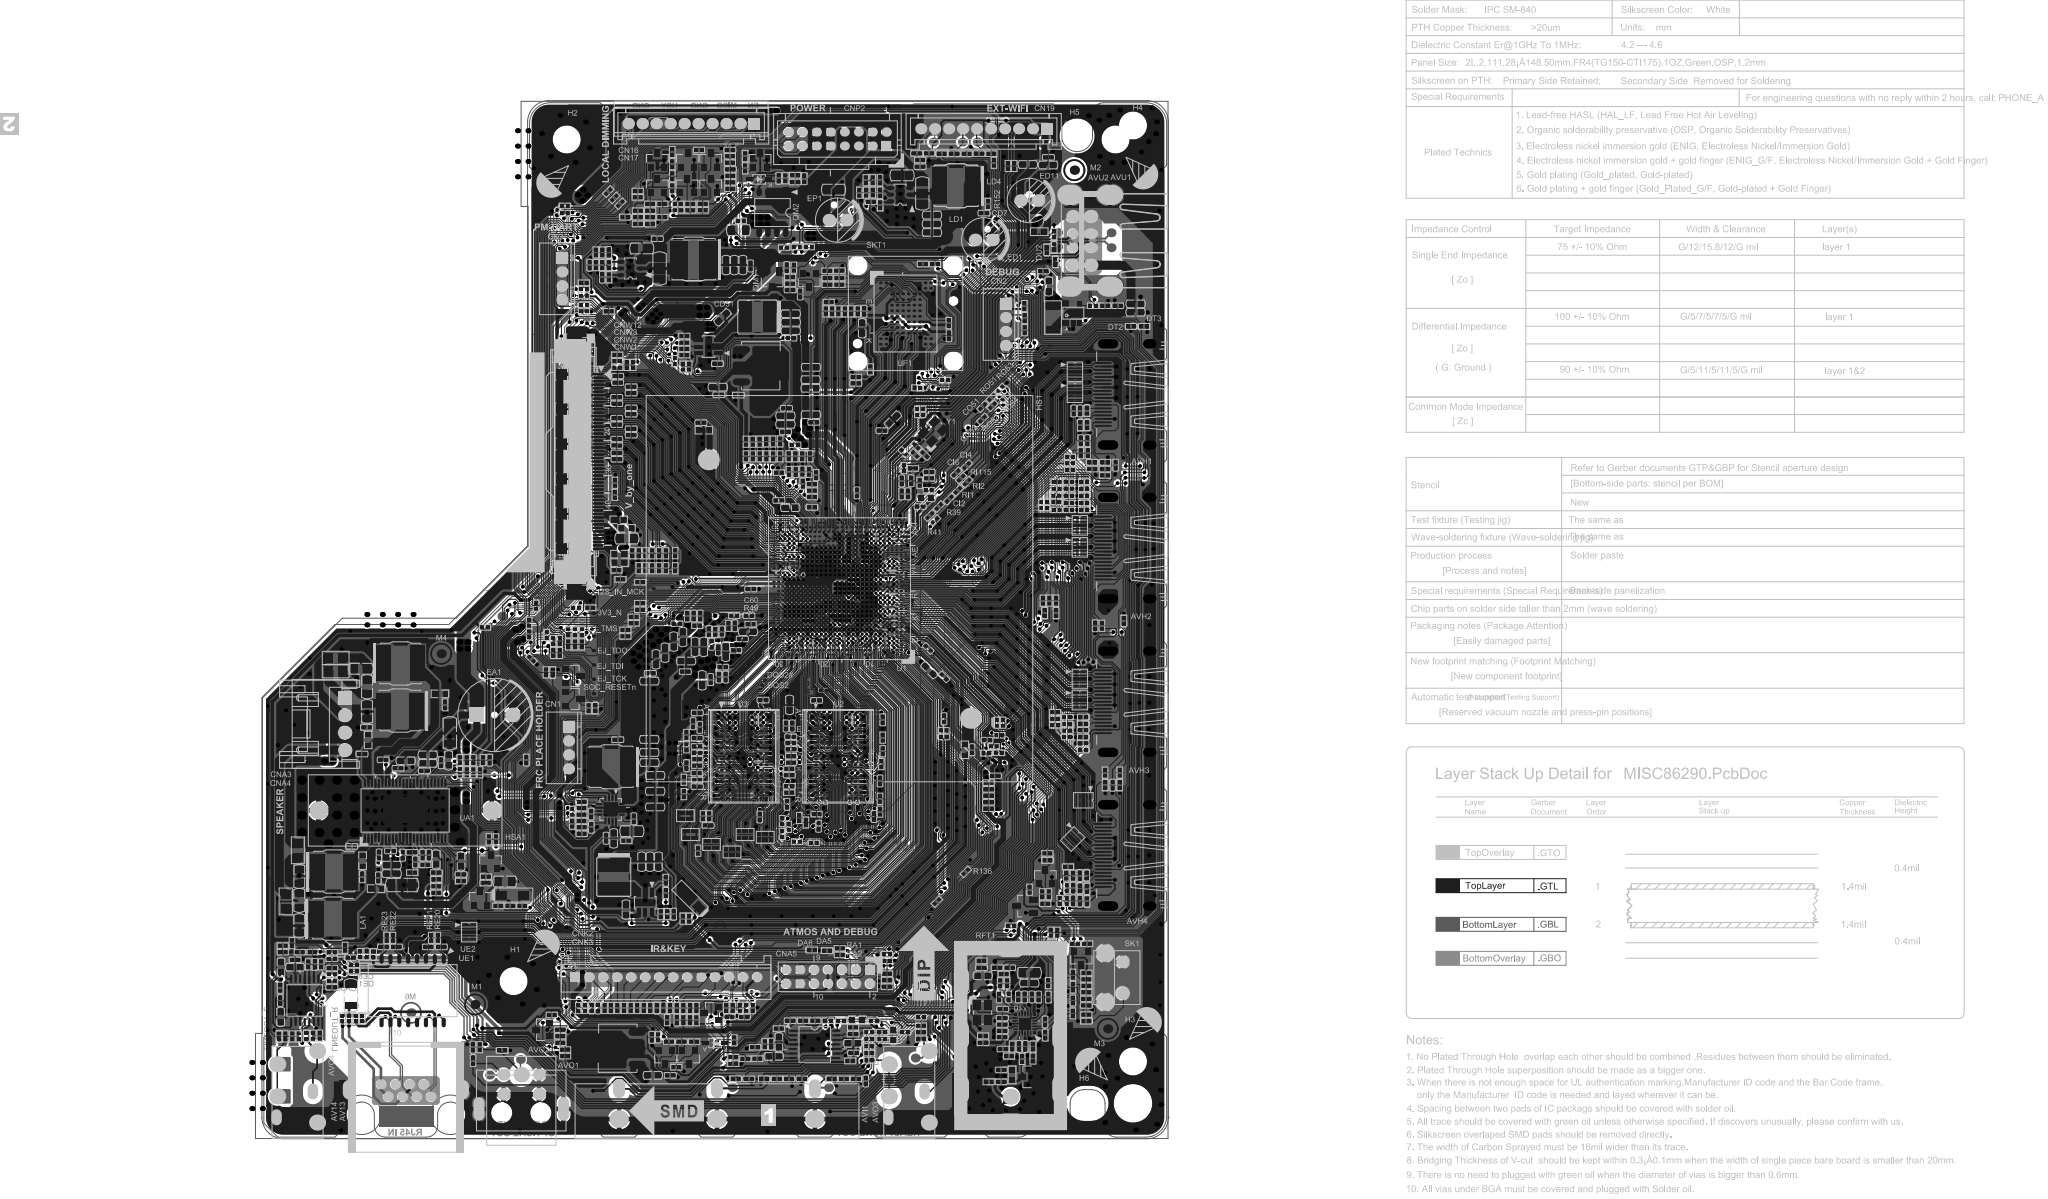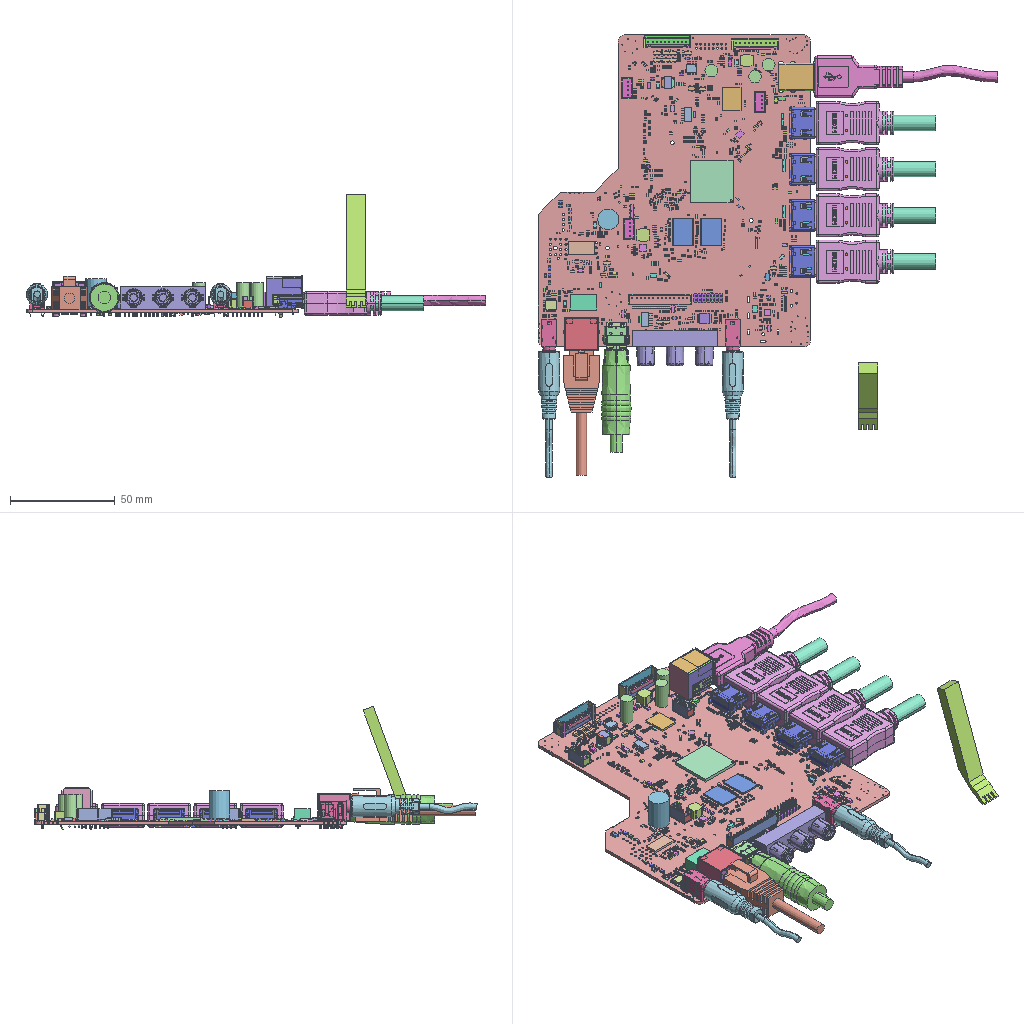Circuit board layout | Altium Designer | box 218.8 x 210.8 x 58.9 mm
Layer stack:
# Altium Designer layer stack of  (unit mm; dielectric type: 0 none, 1 core, 2 prepreg, 3 surface material)
index,name,kind,layer,copper_thickness_mm,dielectric_type,dielectric_thickness_mm,dielectric_material,dielectric_constant
0,TopPaste,other,,,,,,
1,TopOverlay,other,,,,,,
2,TopSolder,dielectric,,,3,0.0102,Solder Resist,3.5
3,TopLayer,copper,TopLayer,0.0356,,,,
4,Dielectric1,dielectric,,,1,1.5,FR-4,4.8
5,BottomLayer,copper,BottomLayer,0.0356,,,,
6,BottomSolder,dielectric,,,3,0.0102,Solder Resist,3.5
7,BottomOverlay,other,,,,,,
8,BottomPaste,other,,,,,,
# drill layer pairs: low layer,high layer
drill_pair,TopLayer,BottomLayer
Part placement, first 372 of 1027 lines:
Designator,Comment,Layer,Footprint,Center-X(mm),Center-Y(mm),Rotation
DH37,NC/TVS diode,DIO ESD,0.5pF,25V,0402 DFN,SMD,AZ5325-01F.R7G,Amazing,TopLayer,DIODE-S0402,-6.316,74.098,270
CH16,22pF-0402-NPO-¡À5%-50V,TopLayer,C0402,-7.493,96.368,90
DBS7,DOLBY PLUS,BottomLayer,DOLBY_PLUS-SILK,-603.079,-354.451,90
CO27,Ceramic capacitor,CAP MC,50V,100pF,¡À5%,NPO,0402,SMD,TP,TopLayer,C0402,-54.026,16.84,360
CO26,Ceramic capacitor,CAP MC,50V,100pF,¡À5%,NPO,0402,SMD,TP,TopLayer,C0402,-45.034,14.91,180
CO15,Ceramic capacitor,CAP MC,50V,680pF,¡À5%,NPO,0402,SMD,TP,Walsin,TopLayer,C0402,-48.628,16.84,180
RU18,4K7ohm-0402-¡À5%-1/16W,TopLayer,R0402,-31.871,108.534,180
RO58,NC/47Kohm-0402-¡À5%-1/16W,TopLayer,R0402,-42.71,14.211,180
RO57,NC/47Kohm-0402-¡À5%-1/16W,TopLayer,R0402,-55.657,15.71,360
RO56,24Kohm-0402-¡À1%-1/16W,TopLayer,R0402,-45.034,15.862,180
RO55,24Kohm-0402-¡À1%-1/16W,TopLayer,R0402,-52.178,16.84,180
RG44,100ohm-0402-¡À5%-1/16W,TopLayer,R0402,-83.547,119.291,360
RG43,100ohm-0402-¡À5%-1/16W,TopLayer,R0402,-75.489,79.616,360
R208,0ohm-0402-¡À5%-1/16W,TopLayer,R0402,-36.194,97.909,315
R207,4K7ohm-0402-¡À5%-1/16W,TopLayer,R0402,-83.845,70.701,90
R206,4K7ohm-0402-¡À5%-1/16W,TopLayer,R0402,-83.845,72.428,270
R205,100ohm-0402-¡À5%-1/16W,TopLayer,R0402,-77.597,71.857,360
R204,100ohm-0402-¡À5%-1/16W,TopLayer,R0402,-77.597,72.784,360
R203,100ohm-0402-¡À5%-1/16W,TopLayer,R0402,-76.423,73.724,360
R202,100ohm-0402-¡À5%-1/16W,TopLayer,R0402,-76.423,74.651,360
R201,100ohm-0402-¡À5%-1/16W,TopLayer,R0402,-75.489,76.606,360
R200,100ohm-0402-¡À5%-1/16W,TopLayer,R0402,-75.495,75.679,360
R31,4K7ohm-0402-¡À5%-1/16W,TopLayer,R0402,-83.553,121.574,0
R30,4K7ohm-0402-¡À5%-1/16W,TopLayer,R0402,-83.553,120.659,0
C14,0.1uF-0402-X5R-¡À20%-16V,TopLayer,C0402,-25.647,47.189,360
M6,MARK,BottomLayer,MARK,-108.28,17.958,180
M5,MARK,BottomLayer,MARK,-13.386,138.608,180
M4,MARK,TopLayer,MARK,-103.95,69.367,0
M3,MARK,TopLayer,MARK,-8.611,15.672,0
M2,MARK,TopLayer,MARK,-13.386,138.608,0
M1,MARK,TopLayer,MARK,-99.111,19.152,0
RT13,NC/0ohm-0402-PCB,TopLayer,R0402SC,-37.782,95.942,270
RT11,NC/0ohm-0402-PCB,TopLayer,R0402SC,-36.462,95.898,180
P1(用于U1上),Thermal grease,0.05g,Other,white,NULL,TopLayer,PCB_TIME,-9.804,-5.969,180
DR4,NC/TVS diode,DIO ESD,3pF,58V,0402,SMD,SDV1005H260C030YPTF,Sunlord,BottomLayer,DIODE-S0402,-37.44,68.694,180
C214,NC/10uF-0805-X5R-¡À20%-16V,BottomLayer,C0805,-55.804,76.327,270
C213,NC/0.1uF-0402-X5R-¡À20%-16V,BottomLayer,C0402,-49.581,77.114,270
C212,NC/0.1uF-0402-X5R-¡À20%-16V,BottomLayer,C0402,-47.625,76.975,270
C211,NC/10uF-0805-X5R-¡À20%-16V,BottomLayer,C0805,-47.676,89.459,225
C210,NC/0.1uF-0402-X5R-¡À20%-16V,BottomLayer,C0402,-46.228,87.122,180
C209,NC/0.1uF-0402-X5R-¡À20%-16V,BottomLayer,C0402,-46.203,88.062,180
C208,NC/10uF-0805-X5R-¡À20%-16V,BottomLayer,C0805,-59.131,73.027,90
C207,NC/0.1uF-0402-X5R-¡À20%-16V,BottomLayer,C0402,-49.454,74.701,135
C206,NC/0.1uF-0402-X5R-¡À20%-16V,BottomLayer,C0402,-50.19,73.254,270
CO25,1uF-0402-X5R-¡À20%-6.3V,TopLayer,C0402,-86.913,15.557,180
5V_M,TEST,BottomLayer,TP,-23.811,124.841,180
CU5,10uF-0603-X5R-¡À20%-6.3V,TopLayer,C0603,-4.623,119.456,360
UH3,Current-limit switch,IC OCP,2.1A,5.5V,H,SOT23-5,SMD,APL3551ABI-TRG,ANPEC,TopLayer,SOT-23-5,-13.538,118.135,360
RU6,4K7ohm-0402-¡À5%-1/16W,TopLayer,R0402,-10.719,119.202,180
RU3,4K7ohm-0402-¡À5%-1/16W,TopLayer,R0402,-8.966,119.202,360
FU1,NC/Resettable fuse,FUSE PTC,1.1A,6V,1206,SMD,TP,TLC,TopLayer,FUSE1.1A-S,-16.434,117.5,270
CU4,0.1uF-0402-X5R-¡À20%-16V,TopLayer,C0402,-17.805,124.155,360
CU3,NC/10uF-0603-X5R-¡À20%-6.3V,TopLayer,C0603,-17.043,121.971,270
CU2,10uF-0603-X5R-¡À20%-6.3V,TopLayer,C0603,-4.623,118.262,360
RM4,1Kohm-0402-¡À5%-1/16W,TopLayer,R0402,-54.038,122.365,360
R73,100ohm-0402-¡À5%-1/16W,TopLayer,R0402,-35.052,125.159,0
R72,100ohm-0402-¡À5%-1/16W,TopLayer,R0402,-33.325,125.171,360
CM4,0.022uF-0402-X7R-¡À10%-16V,TopLayer,C0402,-54.534,124.651,90
RH16,100ohm-0402-¡À5%-1/16W,TopLayer,R0402,-17.678,91.11,180
RH15,100ohm-0402-¡À5%-1/16W,TopLayer,R0402,-17.678,90.195,180
RH14,47Kohm-0402-¡À5%-1/16W,TopLayer,R0402,-15.951,91.11,180
RH13,47Kohm-0402-¡À5%-1/16W,TopLayer,R0402,-15.951,92.024,180
DH14,NC/TVS diode,DIO ESD,0.5pF,25V,0402 DFN,SMD,AZ5325-01F.R7G,Amazing,TopLayer,DIODE-S0402,-11.989,90.957,360
DH13,NC/TVS diode,DIO ESD,0.5pF,25V,0402 DFN,SMD,AZ5325-01F.R7G,Amazing,TopLayer,DIODE-S0402,-11.989,91.999,360
DH12,NC/TVS diode,DIO ESD,0.5pF,25V,0402 DFN,SMD,AZ5325-01F.R7G,Amazing,TopLayer,DIODE-S0402,-11.989,93.015,360
DH11,NC/TVS diode,DIO ESD,0.5pF,25V,0402 DFN,SMD,AZ5325-01F.R7G,Amazing,TopLayer,DIODE-S0402,-11.989,94.005,360
CH14,NC/22pF-0402-NPO-¡À5%-50V,TopLayer,C0402,-14.173,90.958,360
CH13,NC/22pF-0402-NPO-¡À5%-50V,TopLayer,C0402,-14.173,91.999,360
CH12,220pF-0402-NPO-¡À5%-50V,TopLayer,C0402,-14.173,93.015,360
CH11,220pF-0402-NPO-¡À5%-50V,TopLayer,C0402,-14.173,94.006,360
CVBSOUT1,TEST,BottomLayer,TP-20,-33.731,88.29,90
DQS3,TEST,BottomLayer,TP-20,-59.483,59.49,90
DQS3#,TEST,BottomLayer,TP-20,-59.483,60.29,90
DQS2,TEST,TopLayer,TP-20,-58.115,64.846,90
DQS2#,TEST,TopLayer,TP-20,-57.709,65.608,90
DQS1,TEST,BottomLayer,TP-20,-45.983,59.49,90
DQS1#,TEST,BottomLayer,TP-20,-45.983,60.29,90
DQS0,TEST,TopLayer,TP-20,-48.844,64.135,90
DQS0#,TEST,TopLayer,TP-20,-49.733,64.135,90
RR11,33ohm-0402-¡À5%-1/16W,TopLayer,R0402,-62.027,14.021,270
DI1,NC/TVS diode,DIO ESD,3pF,58V,0402,SMD,SDV1005H260C030YPTF,Sunlord,TopLayer,DIODE-S0402,-61.849,8.509,360
AV_L,TEST,BottomLayer,TP,-62.319,7.264,180
RP14,Resistor array,RES ARRAY,1/16W,4¡Á75ohm,¡À5%,0402,SMD,TopLayer,RA0402-MSD6886,-62.358,40.99,270
RK13,NC/33Kohm-0402-¡À5%-1/16W,TopLayer,R0402,-62.268,18.669,270
RO19,NC/?,TopLayer,R0402,-62.172,11.608,180
C59,Ceramic capacitor,CAP MC,50V,1000pF,¡À20%,X7R,0402,SMD,TP,TopLayer,C0402,-61.951,73.391,90
R45,Thick-film resistor,RES,1/16W,10Kohm,¡À5%,0402,SMD,TopLayer,R0402,-62.038,74.829,360
R48,Thick-film resistor,RES,1/16W,240ohm,¡À1%,0402,SMD,TopLayer,R0402,-61.784,69.851,360
MOD_1V2,TEST,BottomLayer,TP,-60.985,94.288,90
U1,TV main chip,IC Main Chip,MSDURN1801-R-00E3,64bit,Multi-Core,BGA758,SMD,Mstar,TopLayer,BGA758/0.65,-46.983,78.69,180
H6,Location hole,TopLayer,ASSE5.0C-3,-5.093,5.292,0
RH38,100ohm-0402-¡À5%-1/16W,TopLayer,R0402,-8.986,52.362,90
DR5,NC/TVS diode,DIO ESD,3pF,58V,0402,SMD,SDV1005H260C030YPTF,Sunlord,TopLayer,DIODE-S0402,-50.902,90.351,180
DH35,NC/TVS diode,DIO ESD,0.5pF,25V,0402 DFN,SMD,AZ5325-01F.R7G,Amazing,TopLayer,DIODE-S0402,-8.973,50.559,90
3V3_STB,TEST,BottomLayer,TP,-94.297,70.968,180
RU5,10Kohm-0402-¡À5%-1/16W,TopLayer,R0402,-51.181,97.638,270
CL25,NC/0.1uF-0402-X5R-¡À20%-16V,TopLayer,C0402,-64.237,106.451,360
CL13,Ceramic capacitor,CAP MC,6.3V,10uF,¡À20%,X5R,0603,SMD,TP,TopLayer,C0603,-64.389,107.544,360
C35,Ceramic capacitor,CAP MC,6.3V,10uF,¡À20%,X5R,0603,SMD,TP,TopLayer,C0603,-54.712,102.21,360
C34,0.1uF-0402-X5R-¡À20%-16V,TopLayer,C0402,-54.572,104.508,180
C33,0.1uF-0402-X5R-¡À20%-16V,TopLayer,C0402,-54.712,101.143,180
C32,0.1uF-0402-X5R-¡À20%-16V,TopLayer,C0402,-53.365,99.289,180
C26,0.1uF-0402-X5R-¡À20%-16V,TopLayer,C0402,-55.651,91.316,180
C25,Ceramic capacitor,CAP MC,6.3V,10uF,¡À20%,X5R,0603,SMD,TP,TopLayer,C0603,-54.026,90.284,360
C20,0.1uF-0402-X5R-¡À20%-16V,TopLayer,C0402,-50.646,102.502,360
MCP_TEST,TEST,BottomLayer,TP-20,-52.172,81.255,180
R26,NC/Thick-film resistor,RES,1/16W,4.7Kohm,¡À5%,0402,SMD,TopLayer,R0402,-59.379,97.627,270
R23,Thick-film resistor,RES,1/16W,4.7Kohm,¡À5%,0402,SMD,TopLayer,R0402,-58.388,97.627,270
R22,Thick-film resistor,RES,1/16W,4.7Kohm,¡À5%,0402,SMD,TopLayer,R0402,-56.458,97.627,270
R21,Thick-film resistor,RES,1/16W,4.7Kohm,¡À5%,0402,SMD,TopLayer,R0402,-60.369,97.627,270
R20,Thick-film resistor,RES,1/16W,4.7Kohm,¡À5%,0402,SMD,TopLayer,R0402,-57.423,97.627,270
R18,Thick-film resistor,RES,1/16W,4.7Kohm,¡À5%,0402,SMD,TopLayer,R0402,-59.404,99.733,90
R15,NC/Thick-film resistor,RES,1/16W,4.7Kohm,¡À5%,0402,SMD,TopLayer,R0402,-58.414,99.733,90
R14,NC/Thick-film resistor,RES,1/16W,4.7Kohm,¡À5%,0402,SMD,TopLayer,R0402,-56.483,99.758,90
R13,NC/Thick-film resistor,RES,1/16W,4.7Kohm,¡À5%,0402,SMD,TopLayer,R0402,-60.369,99.733,90
R12,NC/Thick-film resistor,RES,1/16W,4.7Kohm,¡À5%,0402,SMD,TopLayer,R0402,-57.448,99.758,90
R10,Thick-film resistor,RES,1/16W,4.7Kohm,¡À5%,0402,SMD,TopLayer,R0402,-55.467,97.632,270
R6,NC/Thick-film resistor,RES,1/16W,4.7Kohm,¡À5%,0402,SMD,TopLayer,R0402,-55.467,99.764,90
R27,NC/Thick-film resistor,RES,1/16W,4.7Kohm,¡À5%,0402,SMD,TopLayer,R0402,-52.248,93.726,270
R25,Thick-film resistor,RES,1/16W,4.7Kohm,¡À5%,0402,SMD,TopLayer,R0402,-52.273,95.453,270
R24,Thick-film resistor,RES,1/16W,4.7Kohm,¡À5%,0402,SMD,TopLayer,R0402,-53.264,95.402,270
R19,Thick-film resistor,RES,1/16W,4.7Kohm,¡À5%,0402,SMD,TopLayer,R0402,-50.927,93.65,360
R17,NC/Thick-film resistor,RES,1/16W,4.7Kohm,¡À5%,0402,SMD,TopLayer,R0402,-51.333,95.428,90
R16,NC/Thick-film resistor,RES,1/16W,4.7Kohm,¡À5%,0402,SMD,TopLayer,R0402,-52.299,97.638,90
R11,Thick-film resistor,RES,1/16W,4.7Kohm,¡À5%,0402,SMD,TopLayer,R0402,-50.927,91.821,180
R9,Thick-film resistor,RES,1/16W,4.7Kohm,¡À5%,0402,SMD,TopLayer,R0402,-54.229,95.402,270
R8,NC/Thick-film resistor,RES,1/16W,4.7Kohm,¡À5%,0402,SMD,TopLayer,R0402,-55.651,95.301,360
R7,NC/Thick-film resistor,RES,1/16W,4.7Kohm,¡À5%,0402,SMD,TopLayer,R0402,-50.927,92.735,360
R5,NC/Thick-film resistor,RES,1/16W,4.7Kohm,¡À5%,0402,SMD,TopLayer,R0402,-53.289,97.638,90
R4,Thick-film resistor,RES,1/16W,4.7Kohm,¡À5%,0402,SMD,TopLayer,R0402,-54.254,97.638,90
RO1,100ohm-0402-¡À5%-1/16W,TopLayer,R0402,-24.917,56.096,360
R123,Thick-film resistor,RES,1/16W,1Kohm,¡À5%,0402,SMD,TopLayer,R0402,-32.087,58.395,180
CO3,33pF-0402-NPO-¡À5%-50V,TopLayer,C0402,-25.889,56.998,360
C174,Ceramic capacitor,CAP MC,50V,330pF,¡À5%,NPO,0402,SMD,TP,TopLayer,C0402,-32.087,57.455,180
AV_R,TEST,BottomLayer,TP,-48.539,7.239,180
R118,Thick-film resistor,RES,1/16W,620ohm,¡À1%,0402,SMD,TopLayer,R0402,-55.183,45.407,90
R108,Thick-film resistor,RES,1/16W,10Kohm,¡À5%,0402,SMD,TopLayer,R0402,-54.166,49.49,180
R100,Thick-film resistor,RES,1/16W,240ohm,¡À1%,0402,SMD,TopLayer,R0402,-54.166,52.89,180
R67,Thick-film resistor,RES,1/16W,10Kohm,¡À1%,0402,SMD,TopLayer,R0402,-41.183,48.607,270
R66,Thick-film resistor,RES,1/16W,10Kohm,¡À1%,0402,SMD,TopLayer,R0402,-41.183,46.773,270
R65,Thick-film resistor,RES,1/16W,620ohm,¡À1%,0402,SMD,TopLayer,R0402,-55.183,43.573,90
R64,Thick-film resistor,RES,1/16W,240ohm,¡À1%,0402,SMD,TopLayer,R0402,-40.983,53.573,90
R63,Thick-film resistor,RES,1/16W,10Kohm,¡À5%,0402,SMD,TopLayer,R0402,-50.258,46.398,180
R62,Thick-film resistor,RES,1/16W,10Kohm,¡À5%,0402,SMD,TopLayer,R0402,-40.808,57.357,270
R59,Thick-film resistor,RES,1/16W,75ohm,¡À5%,0402,SMD,TopLayer,R0402,-50.666,42.29,180
R56,Thick-film resistor,RES,1/16W,22ohm,¡À5%,0402,SMD,TopLayer,R0402,-53.066,42.49,180
R55,Thick-film resistor,RES,1/16W,75ohm,¡À5%,0402,SMD,TopLayer,R0402,-52.733,45.857,270
R54,Thick-film resistor,RES,1/16W,75ohm,¡À5%,0402,SMD,TopLayer,R0402,-51.783,45.207,270
R53,Thick-film resistor,RES,1/16W,22ohm,¡À5%,0402,SMD,TopLayer,R0402,-54.262,44.594,270
R52,Thick-film resistor,RES,1/16W,22ohm,¡À5%,0402,SMD,TopLayer,R0402,-40.808,55.407,270
R51,Thick-film resistor,RES,1/16W,22ohm,¡À5%,0402,SMD,TopLayer,R0402,-53.9,53.79,180
R50,Thick-film resistor,RES,1/16W,22ohm,¡À5%,0402,SMD,TopLayer,R0402,-53.9,54.69,180
R49,Thick-film resistor,RES,1/16W,240ohm,¡À1%,0402,SMD,TopLayer,R0402,-59.702,73.61,360
C100,Ceramic capacitor,CAP MC,50V,1000pF,¡À20%,X7R,0402,SMD,TP,TopLayer,C0402,-54.166,51.99,180
C99,Ceramic capacitor,CAP MC,50V,1000pF,¡À20%,X7R,0402,SMD,TP,TopLayer,C0402,-41.183,51.173,90
C98,Ceramic capacitor,CAP MC,50V,1000pF,¡À20%,X7R,0402,SMD,TP,TopLayer,C0402,-53.951,56.59,360
C97,Ceramic capacitor,CAP MC,16V,0.1uF,¡À20%,X5R,0402,SMD,TP,TopLayer,C0402,-49.983,44.673,90
C96,NC/Ceramic capacitor,CAP MC,16V,0.1uF,¡À20%,X5R,0402,SMD,TP,BottomLayer,C0402,-50.383,51.515,270
C95,NC/Ceramic capacitor,CAP MC,16V,0.1uF,¡À20%,X5R,0402,SMD,TP,BottomLayer,C0402,-45.483,56.49,270
C93,NC/Ceramic capacitor,CAP MC,16V,0.1uF,¡À20%,X5R,0402,SMD,TP,BottomLayer,C0402,-57.683,54.965,90
C92,NC/Ceramic capacitor,CAP MC,16V,0.1uF,¡À20%,X5R,0402,SMD,TP,BottomLayer,C0402,-57.683,57.065,90
C91,NC/Ceramic capacitor,CAP MC,16V,0.1uF,¡À20%,X5R,0402,SMD,TP,BottomLayer,C0402,-57.651,50.665,90
C90,NC/Ceramic capacitor,CAP MC,16V,0.1uF,¡À20%,X5R,0402,SMD,TP,BottomLayer,C0402,-49.74,49.203,180
C83,NC/Ceramic capacitor,CAP MC,16V,0.1uF,¡À20%,X5R,0402,SMD,TP,BottomLayer,C0402,-58.283,48.673,90
C76,Ceramic capacitor,CAP MC,16V,0.1uF,¡À20%,X5R,0402,SMD,TP,TopLayer,C0402,-57.916,62.74,180
C74,Ceramic capacitor,CAP MC,16V,0.1uF,¡À20%,X5R,0402,SMD,TP,TopLayer,C0402,-42.058,46.073,90
C73,Ceramic capacitor,CAP MC,16V,0.1uF,¡À20%,X5R,0402,SMD,TP,TopLayer,C0402,-53.9,55.69,360
C70,Ceramic capacitor,CAP MC,16V,0.1uF,¡À20%,X5R,0402,SMD,TP,TopLayer,C0402,-40.808,59.923,90
C67,Ceramic capacitor,CAP MC,16V,0.1uF,¡À20%,X5R,0402,SMD,TP,TopLayer,C0402,-50.266,62.69,180
C66,Ceramic capacitor,CAP MC,16V,0.1uF,¡À20%,X5R,0402,SMD,TP,TopLayer,C0402,-53.73,59.028,90
C65,Ceramic capacitor,CAP MC,16V,0.1uF,¡À20%,X5R,0402,SMD,TP,TopLayer,C0402,-54.633,59.028,90
C60,Ceramic capacitor,CAP MC,16V,0.1uF,¡À20%,X5R,0402,SMD,TP,TopLayer,C0402,-59.949,74.817,180
C58,NC/Ceramic capacitor,CAP MC,16V,0.1uF,¡À20%,X5R,0402,SMD,TP,TopLayer,C0402,-60.884,71.488,360
C51,Ceramic capacitor,CAP MC,6.3V,10uF,¡À20%,X5R,0603,SMD,TP,TopLayer,C0603,-54.128,62.051,270
C50,Ceramic capacitor,CAP MC,6.3V,0.47uF,¡À10%,X5R,0402,SMD,TP,TopLayer,C0402,-58.393,45.993,270
C46,NC/Ceramic capacitor,CAP MC,6.3V,0.47uF,¡À10%,X5R,0402,SMD,TP,BottomLayer,C0402,-45.866,73.49,360
C42,0.1uF-0402-X5R-¡À20%-16V,TopLayer,C0402,-54.483,47.807,90
C39,Ceramic capacitor,CAP MC,6.3V,10uF,¡À20%,X5R,0603,SMD,TP,TopLayer,C0603,-60.071,72.53,360
UH22,NC/TVS diode,DIO ESD,0.4pF,19V,DFN2510-10L,SMD,ESD5304D-10/TR,Willsemi,TopLayer,RCL0524P,-12.598,62.738,270
UA2,Audio amplifier,IC Headphone AMP,Class AB,2¡Á20mW@2.3V@32ohm,TSSOP-14,SMD,AD22653B-QH14NAR,ESMT,TopLayer,SSOP14/0.65-1,-50.521,13.437,270
RO30,4K7ohm-0402-¡À5%-1/16W,TopLayer,R0402,-59.055,13.03,360
RO29,0ohm-0402-¡À5%-1/16W,TopLayer,R0402,-57.683,13.462,90
RO25,1Kohm-0402-¡À5%-1/16W,TopLayer,R0402,-42.71,12.192,360
RO24,1Kohm-0402-¡À5%-1/16W,TopLayer,R0402,-35.316,15.186,360
RO23,10Kohm-0402-¡À5%-1/16W,TopLayer,R0402,-86.226,12.7,180
RO22,1Kohm-0402-¡À5%-1/16W,TopLayer,R0402,-88.145,17.653,360
RO21,30Kohm-0402-¡À1%-1/16W,TopLayer,R0402,-58.725,11.405,360
RO20,1Kohm-0402-¡À5%-1/16W,TopLayer,R0402,-60.445,11.379,360
RO16,5R1ohm-0402-¡À5%-1/16W,TopLayer,R0402,-42.71,13.157,360
RO15,5R1ohm-0402-¡À5%-1/16W,TopLayer,R0402,-35.316,16.138,360
RO14,10Kohm-0402-¡À5%-1/16W,TopLayer,R0402,-42.71,15.186,180
RO12,10Kohm-0402-¡À5%-1/16W,TopLayer,R0402,-40.856,14.211,180
RO11,10Kohm-0402-¡À5%-1/16W,TopLayer,R0402,-46.749,16.84,180
RK23,22ohm-0402-¡À5%-1/16W,TopLayer,R0402,-62.713,17.374,360
RK14,NC/510ohm-0402-¡À1%-1/16W,TopLayer,R0402,-61.227,18.682,90
LO2,Ferrite bead,BEAD,120ohm,0402,500mA,SMD,TP,GZ1005U121CTF,Sunlord,TopLayer,L0402,-45.441,11.074,180
H3,Location hole,TopLayer,ASSE3.5C-3,-5.1,8.216,0
DO12,NC/NC?,TopLayer,DIODE-S0402,-42.697,11.176,360
DO11,NC/NC?,TopLayer,DIODE-S0402,-35.306,14.211,360
CO24,NC/0.1uF-0402-X5R-¡À20%-16V,TopLayer,C0402,-91.77,54.14,90
CO21,0.1uF-0402-X5R-¡À20%-16V,TopLayer,C0402,-44.958,12.217,360
CO20,10uF-0603-X5R-¡À20%-6.3V,TopLayer,C0603,-45.034,13.589,360
CO19,10uF-0603-X5R-¡À20%-6.3V,TopLayer,C0603,-56.388,11.709,180
CO18,0.1uF-0402-X5R-¡À20%-16V,TopLayer,C0402,-56.744,13.462,90
CO16,Ceramic capacitor,CAP MC,50V,680pF,¡À5%,NPO,0402,SMD,TP,Walsin,TopLayer,C0402,-40.85,15.185,180
CO14,Ceramic capacitor,CAP MC,6.3V,10uF,¡À20%,X5R,0603,SMD,TP,TopLayer,C0603,-39.256,14.757,90
CO13,Ceramic capacitor,CAP MC,6.3V,10uF,¡À20%,X5R,0603,SMD,TP,TopLayer,C0603,-44.417,16.98,360
CO12,NC/000pF-0402-X7R-¡À10%-50V,TopLayer,C0402,-37.599,15.185,180
CO11,NC/1000pF-0402-X7R-¡À10%-50V,TopLayer,C0402,-42.031,16.841,360
CNA5,Gold-plated pin,pin connector,2¡Á7Pin,D,D2.0,L=2.6mm,DIP,LD,TopLayer,SIP2*7/2.0D,-48.641,23.13,360
CK8,Ceramic capacitor,CAP MC,50V,1000pF,¡À20%,X7R,0402,SMD,TP,TopLayer,C0402,-60.579,17.374,180
CK7,NC/1000pF-0402-X7R-¡À10%-50V,TopLayer,C0402,-59.411,18.682,90
C24,1uF-0402-X5R-¡À20%-6.3V,TopLayer,C0402,-32.017,66.065,315
U2,DDR chip,IC DDR3,DDR3,2133M,16bit,256MB,2Gb,FBGA96,SMD,K4B2G1646F-BCNB,Samsung,TopLayer,BGA96/0.8-1,-47.183,54.69,360
RP16,Resistor array,RES ARRAY,1/16W,4¡Á75ohm,¡À5%,0402,SMD,TopLayer,RA0402-MSD6886,-57.608,43.09,270
RP13,Resistor array,RES ARRAY,1/16W,4¡Á75ohm,¡À5%,0402,SMD,TopLayer,RA0402-MSD6886,-60.483,43.49,270
C85,NC/Ceramic capacitor,CAP MC,16V,0.1uF,¡À20%,X5R,0402,SMD,TP,BottomLayer,C0402,-42.266,58.309,180
C88,NC/Ceramic capacitor,CAP MC,16V,0.1uF,¡À20%,X5R,0402,SMD,TP,BottomLayer,C0402,-41.516,49.19,180
C81,Ceramic capacitor,CAP MC,16V,0.1uF,¡À20%,X5R,0402,SMD,TP,TopLayer,C0402,-54.166,50.39,180
C82,Ceramic capacitor,CAP MC,16V,0.1uF,¡À20%,X5R,0402,SMD,TP,TopLayer,C0402,-53.951,57.5,360
QO21,General-purpose transistor,Dynatron,NPN,0.2A,40V,60-300,SOT-23,KMBT3904,KEXIN,TopLayer,SOT-23,-89.472,15.545,270
RO26,10Kohm-0402-¡À5%-1/16W,TopLayer,R0402,-35.306,17.335,360
RO27,4K7ohm-0402-¡À5%-1/16W,TopLayer,R0402,-86.913,14.618,360
RO28,NC/?,TopLayer,R0402,-86.913,13.679,180
CI1,NC/56pF-0402-NPO-¡À5%-50V,TopLayer,C0402,-59.969,8.509,180
CI3,NC/56pF-0402-NPO-¡À5%-50V,TopLayer,C0402,-52.356,8.509,180
CI5,NC/56pF-0402-NPO-¡À5%-50V,TopLayer,C0402,-43.231,8.204,90
DI2,NC/TVS diode,DIO ESD,3pF,58V,0402,SMD,SDV1005H260C030YPTF,Sunlord,TopLayer,DIODE-S0402,-57.76,8.509,360
DI3,NC/TVS diode,DIO ESD,3pF,58V,0402,SMD,SDV1005H260C030YPTF,Sunlord,TopLayer,DIODE-S0402,-48.082,8.509,180
RI3,10Kohm-0402-¡À5%-1/16W,TopLayer,R0402,-55.931,8.509,360
RI4,18Kohm-0402-¡À1%-1/16W,TopLayer,R0402,-54.185,8.509,180
RI5,18Kohm-0402-¡À1%-1/16W,TopLayer,R0402,-44.628,8.509,180
RI6,10Kohm-0402-¡À5%-1/16W,TopLayer,R0402,-46.355,8.509,360
YT2,24MHz-¡À20ppm-16pF-3.2*2.5-SMD,TopLayer,XTAL-S-3,-26.518,17.983,270
DT3,NC/TVS diode,DIO ESD,3pF,58V,0402,SMD,SDV1005H260C030YPTF,Sunlord,TopLayer,DIODE-S0402,-3.404,116.23,180
DT2,NC/TVS diode,DIO ESD,3pF,58V,0402,SMD,SDV1005H260C030YPTF,Sunlord,TopLayer,DIODE-S0402,-5.283,116.23,360
CT40,Ceramic capacitor,CAP MC,50V,12pF,¡À5%,NPO,0402,SMD,TP,TopLayer,C0402,-23.682,17.218,360
CT39,Ceramic capacitor,CAP MC,50V,12pF,¡À5%,NPO,0402,SMD,TP,TopLayer,C0402,-23.645,18.502,180
3V3_Tun,TEST,BottomLayer,TP,-39.802,18.136,315
CH15,22pF-0402-NPO-¡À5%-50V,TopLayer,C0402,-7.925,50.546,90
CH21,220pF-0402-NPO-¡À5%-50V,TopLayer,C0402,-14.376,57.455,360
CH22,220pF-0402-NPO-¡À5%-50V,TopLayer,C0402,-12.141,56.54,180
CH23,NC/22pF-0402-NPO-¡À5%-50V,TopLayer,C0402,-12.141,58.42,180
CH24,NC/22pF-0402-NPO-¡À5%-50V,TopLayer,C0402,-14.376,60.3,360
CH31,220pF-0402-NPO-¡À5%-50V,TopLayer,C0402,-12.598,33.941,270
CH32,220pF-0402-NPO-¡À5%-50V,TopLayer,C0402,-13.564,33.985,90
CH33,NC/22pF-0402-NPO-¡À5%-50V,TopLayer,C0402,-13.538,35.814,270
CH34,NC/22pF-0402-NPO-¡À5%-50V,TopLayer,C0402,-12.598,37.617,270
CR1,1uF-0402-X5R-¡À20%-6.3V,TopLayer,C0402,-11.671,19.952,360
CR2,0.1uF-0402-X5R-¡À20%-16V,TopLayer,C0402,-22.428,30.429,360
CR3,0.1uF-0402-X5R-¡À20%-16V,TopLayer,C0402,-13.589,21.615,90
CR4,0.1uF-0402-X5R-¡À20%-16V,TopLayer,C0402,-11.671,19.012,180
DH21,NC/TVS diode,DIO ESD,0.5pF,25V,0402 DFN,SMD,AZ5325-01F.R7G,Amazing,TopLayer,DIODE-S0402,-12.141,55.601,360
DH22,NC/TVS diode,DIO ESD,0.5pF,25V,0402 DFN,SMD,AZ5325-01F.R7G,Amazing,TopLayer,DIODE-S0402,-12.141,57.429,360
DH23,NC/TVS diode,DIO ESD,0.5pF,25V,0402 DFN,SMD,AZ5325-01F.R7G,Amazing,TopLayer,DIODE-S0402,-12.141,59.334,360
DH24,NC/TVS diode,DIO ESD,0.5pF,25V,0402 DFN,SMD,AZ5325-01F.R7G,Amazing,TopLayer,DIODE-S0402,-12.141,60.3,360
DH31,NC/TVS diode,DIO ESD,0.5pF,25V,0402 DFN,SMD,AZ5325-01F.R7G,Amazing,TopLayer,DIODE-S0402,-11.582,35.738,270
DH32,NC/TVS diode,DIO ESD,0.5pF,25V,0402 DFN,SMD,AZ5325-01F.R7G,Amazing,TopLayer,DIODE-S0402,-11.582,33.934,270
DH33,NC/TVS diode,DIO ESD,0.5pF,25V,0402 DFN,SMD,AZ5325-01F.R7G,Amazing,TopLayer,DIODE-S0402,-12.573,35.763,90
DH34,NC/TVS diode,DIO ESD,0.5pF,25V,0402 DFN,SMD,AZ5325-01F.R7G,Amazing,TopLayer,DIODE-S0402,-11.633,37.617,90
DH36,NC/TVS diode,DIO ESD,0.5pF,25V,0402 DFN,SMD,AZ5325-01F.R7G,Amazing,TopLayer,DIODE-S0402,-6.909,50.559,90
DR2,TVS diode,DIO ESD,3pF,58V,0402,SMD,SDV1005H260C030YPTF,Sunlord,TopLayer,DIODE-S0402,-11.671,16.777,360
QR1,KMBT3906,TopLayer,SOT-23,-12.421,25.806,360
R153,4K7ohm-0402-¡À5%-1/16W,TopLayer,R0402,-13.303,27.864,360
RH21,Thick-film resistor,RES,1/16W,33ohm,¡À5%,0402,SMD,TopLayer,R0402,-16.129,59.131,360
RH23,47Kohm-0402-¡À5%-1/16W,TopLayer,R0402,-14.376,58.369,360
RH24,47Kohm-0402-¡À5%-1/16W,TopLayer,R0402,-14.376,59.284,360
RH25,100ohm-0402-¡À5%-1/16W,TopLayer,R0402,-16.129,60.985,180
RH26,100ohm-0402-¡À5%-1/16W,TopLayer,R0402,-16.129,60.071,180
RH31,Thick-film resistor,RES,1/16W,33ohm,¡À5%,0402,SMD,TopLayer,R0402,-15.494,33.985,270
RH32,Thick-film resistor,RES,1/16W,33ohm,¡À5%,0402,SMD,TopLayer,R0402,-14.503,33.985,90
RH33,47Kohm-0402-¡À5%-1/16W,TopLayer,R0402,-14.529,37.617,90
RH34,47Kohm-0402-¡À5%-1/16W,TopLayer,R0402,-13.564,37.592,270
RH35,100ohm-0402-¡À5%-1/16W,TopLayer,R0402,-14.3,38.887,180
RH36,100ohm-0402-¡À5%-1/16W,TopLayer,R0402,-14.503,35.814,270
RH37,100ohm-0402-¡À5%-1/16W,TopLayer,R0402,-6.909,52.362,90
RR3,4K7ohm-0402-¡À5%-1/16W,TopLayer,R0402,-13.589,23.419,90
RR4,2K2ohm-0402-¡À5%-1/16W,TopLayer,R0402,-11.557,27.864,360
RR5,100ohm-0402-¡À5%-1/16W,TopLayer,R0402,-11.659,21.823,180
RR7,10Kohm-0402-¡À5%-1/16W,TopLayer,R0402,-11.659,22.737,180
RR8,100ohm-0402-¡À5%-1/16W,TopLayer,R0402,-11.671,20.892,180
RR9,4K7ohm-0402-¡À5%-1/16W,TopLayer,R0402,-11.659,23.673,180
RR10,33ohm-0402-¡À5%-1/16W,TopLayer,R0402,-11.671,17.716,360
UH31,NC/TVS diode,DIO ESD,0.4pF,19V,DFN2510-10L,SMD,ESD5304D-10/TR,Willsemi,TopLayer,RCL0524P,-12.097,48.386,180
UH32,NC/TVS diode,DIO ESD,0.4pF,19V,DFN2510-10L,SMD,ESD5304D-10/TR,Willsemi,TopLayer,RCL0524P,-13.629,42.86,225
RT5,4K7ohm-0402-¡À5%-1/16W,TopLayer,R0402,-15.812,29.433,90
RT9,100ohm-0402-¡À5%-1/16W,TopLayer,R0402,-17.12,22.212,90
CT10,0.1uF-0402-X5R-¡À20%-16V,TopLayer,C0402,-17.094,20.218,90
CT28,NC/0.1uF-0805-X7R-¡À10%-50V,TopLayer,C0805,-19.832,23.688,180
RT4,Ferrite bead,BEAD,120ohm,0402,500mA,SMD,TP,GZ1005U121CTF,Sunlord,TopLayer,L0402,-26.441,14.656,360
CT30,10uF-0603-X5R-¡À20%-6.3V,TopLayer,C0603,-19.833,22.215,180
CT8,33pF-0402-NPO-¡À5%-50V,TopLayer,C0402,-22.805,20.234,270
CT7,33pF-0402-NPO-¡À5%-50V,TopLayer,C0402,-24.151,20.234,90
CT5,22pF-0402-NPO-¡À5%-50V,TopLayer,C0402,-17.577,16.65,90
CT3,10uF-0603-X5R-¡À20%-6.3V,TopLayer,C0603,-26.492,23.266,180
CT1,Ceramic capacitor,CAP MC,50V,1000pF,¡À20%,X7R,0402,SMD,TP,TopLayer,C0402,-23.699,14.482,360
CT2,Ceramic capacitor,CAP MC,50V,1000pF,¡À20%,X7R,0402,SMD,TP,TopLayer,C0402,-23.58,12.78,360
CT9,30pF-0402-NPO-¡À5%-50V,TopLayer,C0402,-20.393,13.141,270
CT15,1uF-0402-X5R-¡À20%-6.3V,TopLayer,C0402,-23.699,15.371,180
CT16,1uF-0402-X5R-¡À20%-6.3V,TopLayer,C0402,-19.457,20.231,270
CT17,Ceramic capacitor,CAP MC,50V,1000pF,¡À20%,X7R,0402,SMD,TP,TopLayer,C0402,-18.501,20.221,270
CT19,Ceramic capacitor,CAP MC,50V,1000pF,¡À20%,X7R,0402,SMD,TP,TopLayer,C0402,-23.699,16.285,360
CT20,Ceramic capacitor,CAP MC,50V,1000pF,¡À20%,X7R,0402,SMD,TP,TopLayer,C0402,-20.493,20.234,270
CT24,NC/180pF-0402-NPO-¡À5%-50V,TopLayer,C0402,-23.843,9.787,180
CT25,Ceramic capacitor,CAP MC,50V,1000pF,¡À20%,X7R,0402,SMD,TP,TopLayer,C0402,-23.843,8.085,360
DT1,Switching diode,DIO SW D2,75V,SOT-23,SMD,KAV99,KEXIN,TopLayer,SO-23,-19.86,8.792,270
LT3,0ohm-0402-¡À5%-1/16W,TopLayer,L0402,-22.731,11.764,180
LT4,SDCL1005CR33JTDF,TopLayer,L0402,-25.646,8.085,180
LT5,SDCL1005CR33JTDF,TopLayer,L0402,-22.273,13.141,270
LT6,SDCL1005CR33JTDF,TopLayer,L0402,-19.302,13.141,270
LT7,0ohm-0402-¡À5%-1/16W,TopLayer,L0402,-19.309,11.417,270
LT9,NC/Multilayer inductor,HF Inductor,180nH,¡À5%,0603,SMD,SDCL1608CR18JTDF,Sunlord,TopLayer,L0603,-22.294,9.075,90
NC/ESD,NC/ESD,TopLayer,ESD,-23.533,4.94,225
RT3,0ohm-0402-¡À5%-1/16W,TopLayer,R0402,-20.851,11.363,90
RT10,100ohm-0402-¡À5%-1/16W,TopLayer,R0402,-23.973,22.19,90
RT12,100ohm-0402-¡À5%-1/16W,TopLayer,R0402,-23.008,22.183,90
CT23,30pF-0402-NPO-¡À5%-50V,TopLayer,C0402,-21.308,13.141,270
CT4,22pF-0402-NPO-¡À5%-50V,TopLayer,C0402,-17.551,14.77,270
UT2,Silicon RF tuner,IC Si Tuner,QFN-24,SMD,SI2151-A10-GMR,Silicon Labs,TopLayer,QFN24/0.4-1,-20.444,16.418,180
CT26,22pF-0402-NPO-¡À5%-50V,TopLayer,C0402,-26.441,13.691,360
RT8,100ohm-0402-¡À5%-1/16W,TopLayer,R0402,-13.602,17.869,90
CT21,NC/47pF-0402-NPO-¡À5%-50V,TopLayer,C0402,-22.652,24.425,360
LT10,NC/,TopLayer,R0402,-23.49,23.51,360
CT6,NC/47pF-0402-NPO-¡À5%-50V,TopLayer,C0402,-24.43,24.425,360
CT31,1uF-0402-X5R-¡À20%-6.3V,TopLayer,C0402,-21.408,20.234,270
CT33,0.1uF-0402-X5R-¡À20%-16V,TopLayer,C0402,-26.67,24.409,180
FT1,Ferrite bead,BEAD,120ohm,0402,500mA,SMD,TP,GZ1005U121CTF,Sunlord,TopLayer,L0402,-26.67,25.4,360
RT2,100ohm-0402-¡À5%-1/16W,TopLayer,R0402,-13.602,19.729,90
RT6,4K7ohm-0402-¡À5%-1/16W,TopLayer,R0402,-16.777,29.443,90
C13,0.1uF-0402-X5R-¡À20%-16V,TopLayer,C0402,-32.022,60.058,270
C201,NC/PZ1608U121-2R0TF(120ohm-2000mA),TopLayer,R0603,-29.058,55.626,90
C205,NC/?,TopLayer,C0402,-28.016,55.626,90
RO2,NC/120ohm-0402-¡À5%-1/16W,TopLayer,R0402,-24.175,55.194,180
RU1,0ohm-0402-¡À5%-1/16W,TopLayer,R0402,-24.501,59.506,270
RU2,0ohm-0402-¡À5%-1/16W,TopLayer,R0402,-23.579,59.506,270
C12,Ceramic capacitor,CAP MC,6.3V,10uF,¡À20%,X5R,0603,SMD,TP,TopLayer,C0603,-34.125,67.031,135
C15,0.1uF-0402-X5R-¡À20%-16V,TopLayer,C0402,-25.647,48.122,0
C27,0.1uF-0402-X5R-¡À20%-16V,TopLayer,C0402,-25.647,49.047,360
C28,0.1uF-0402-X5R-¡À20%-16V,TopLayer,C0402,-25.647,49.962,360
C29,NC/0.1uF-0402-X5R-¡À20%-16V,BottomLayer,C0402,-42.774,73.482,180
C30,1uF-0402-X5R-¡À20%-6.3V,TopLayer,C0402,-24.687,51.88,180
C111,1uF-0402-X5R-¡À20%-6.3V,TopLayer,C0402,-34.294,70.133,135
CA29,NC/Ceramic capacitor,CAP MC,50V,1000pF,¡À10%,X7R,0402,SMD,TP,TopLayer,C0402,-40.183,21.717,360
CN2,Connector socket,connect jack,4Pin,D2.0,D,Beige,L=2.8mm,DIP,W2011-04SVA-SN8-ENSY,XYDT,TopLayer,SIP4/2.0D-1,-23.216,116.51,270
D40,NC/SFI0402-240E-2R5PP-LF,TopLayer,DIODE-S0402,-17.653,75.184,90
D41,NC/SFI0402-240E-2R5PP-LF,TopLayer,DIODE-S0402,-16.002,75.184,90
DA1,NC/AVLC18S02003,TopLayer,DIODE-S0402,-40.183,22.631,360
DA2,NC/AVLC18S02003,TopLayer,DIODE-S0402,-40.183,26.34,180
DA5,NC/AVLC18S02003,TopLayer,DIODE-S0402,-48.768,26.873,360
DA6,NC/AVLC18S02003,TopLayer,DIODE-S0402,-50.927,26.949,180
DR1,NC/TVS diode,DIO ESD,3pF,58V,0402,SMD,SDV1005H260C030YPTF,Sunlord,TopLayer,DIODE-S0402,-17.234,39.789,360
QR4,General-purpose transistor,Dynatron,NPN,0.2A,40V,60-300,SOT-23,KMBT3904,KEXIN,TopLayer,SOT-23,-17.541,37.465,180
R3,0ohm-0402-¡À5%-1/16W,TopLayer,R0402,-25.647,50.923,360
R135,0ohm-0402-¡À5%-1/16W,TopLayer,R0402,-33.045,33.884,225
R136,0ohm-0402-¡À5%-1/16W,TopLayer,R0402,-28.918,38.151,225
R137,0ohm-0402-¡À5%-1/16W,TopLayer,R0402,-20.523,119.151,90
R138,4K7ohm-0402-¡À5%-1/16W,TopLayer,R0402,-20.498,115.697,90
R139,4K7ohm-0402-¡À5%-1/16W,TopLayer,R0402,-20.498,117.424,270
R140,100ohm-0402-¡À5%-1/16W,TopLayer,R0402,-16.002,76.987,270
R141,100ohm-0402-¡À5%-1/16W,TopLayer,R0402,-17.882,76.975,270
R151,4K7ohm-0402-¡À5%-1/16W,TopLayer,R0402,-24.099,57.691,360
RA1,22ohm-0402-¡À5%-1/16W,TopLayer,R0402,-46.939,27.178,180
RA2,22ohm-0402-¡À5%-1/16W,TopLayer,R0402,-46.939,26.264,180
RA3,22ohm-0402-¡À5%-1/16W,TopLayer,R0402,-40.183,25.4,180
RA4,22ohm-0402-¡À5%-1/16W,TopLayer,R0402,-40.183,23.571,360
RR1,1Kohm-0402-¡À5%-1/16W,TopLayer,R0402,-17.971,34.925,270
RR2,10Kohm-0402-¡À5%-1/16W,TopLayer,R0402,-19.799,35.592,90
RR17,10Kohm-0402-¡À5%-1/16W,TopLayer,R0402,-17.234,40.78,180
RR18,NC/0ohm-0402-¡À5%-1/16W,TopLayer,R0402,-17.043,34.925,90
RR19,NC/,TopLayer,R0402,-17.546,33.592,360
UR1,Reset IC,IC Reset,LOW,2.93V,SOT-23,SMD,SGM803-SXN3L/TR,SGMICRO,TopLayer,SOT-23-3-1,-20.434,33.236,90
Pad and via stacks, first 71 of 218 lines:
# Altium Designer via and pad stacks of  (unit mm). Each distinct definition once, with the count of objects using it.
# via: kind,start_layer,end_layer,hole_mm,diameter_mm,mode(0 simple;1 top-mid-bottom;2 full stack),diameter_per_layer,count,example_net
# pad: kind,layer,hole_mm,hole_type(0 round;1 square;2 slot),plating,top_size,top_shape(1 round;2 rect;3 octagon;9 rounded rect),mid_size,bottom_size,mode,footprint,size_per_layer,count,example
pad,3D\u00BA\u00CD\u00D7\u00B0\u00C5\u00E4,0,0,unplated,0.3x0.3,1,0.3x0.3,0.3x0.3,0,Barcode,,3,S/N1.0
pad,3D\u00BA\u00CD\u00D7\u00B0\u00C5\u00E4,0,0,unplated,0.3x0.3,1,0.3x0.3,0.3x0.3,0,Manufacture_Info,,1,Manufacture_Info.0
pad,3D\u00BA\u00CD\u00D7\u00B0\u00C5\u00E4,0,0,unplated,0.3x0.3,1,0.3x0.3,0.3x0.3,0,PCB_TIME,,2,P1(\u00D3\u00C3\u00D3\u00DAU1\u00C9\u00CF).0
pad,3D\u00BA\u00CD\u00D7\u00B0\u00C5\u00E4,0,0,unplated,0.3x0.3,1,0.3x0.3,0.3x0.3,0,PCB_NAME,,1,XXXXXXXXXXX.0
pad,MultiLayer,0.5,0,plated,0.8x0.8,1,0.8x0.8,0.8x0.8,0,,,70,VIA5
pad,MultiLayer,0.2,0,plated,0.4x0.4,1,0.4x0.4,0.4x0.4,0,,,57,VIA5
pad,MultiLayer,0.4064,0,plated,0.6096x0.6096,1,1.524x1.524,0.6096x0.6096,1,,,4,VIA5
pad,MultiLayer,0.4,0,plated,0.6x0.6,1,0.6x0.6,0.6x0.6,0,,,60,VIA5
pad,MultiLayer,0.8,0,plated,1.1x1.1,2,1.1x1.1,1.1x1.1,0,SIP4/2.0D-1,,3,CN3.1
pad,MultiLayer,0.8,0,plated,1.1x1.1,1,1.1x1.1,1.1x1.1,0,SIP4/2.0D-1,,9,CN3.2
pad,MultiLayer,0.4,0,plated,0.7x0.7,1,0.7x0.7,0.7x0.7,0,ASSE5.0C-3,,6,H6.2
pad,MultiLayer,0.4,0,plated,0.7x0.7,1,0.7x0.7,0.7x0.7,0,ASSE3.5C-3,,30,H3.2
pad,MultiLayer,0.8,0,plated,1.1x1.1,1,1.1x1.1,1.1x1.1,0,SIP2*7/2.0D,,14,CNA5.11
pad,MultiLayer,0.8,0,plated,1.1x1.1,1,1.1x1.1,1.1x1.1,0,SIP2*8/2.0D-5,,15,CNP2.12
pad,MultiLayer,0.8,0,plated,1.1x1.1,2,1.1x1.1,1.1x1.1,0,SIP2*8/2.0D-5,,1,CNP2.1
pad,MultiLayer,0.8,0,plated,1.1x1.1,2,1.1x1.1,1.1x1.1,0,SIP10/2.0D-4,,2,CN19.1
pad,MultiLayer,0.8,0,plated,1.1x1.1,1,1.1x1.1,1.1x1.1,0,SIP10/2.0D-4,,18,CN19.2
pad,MultiLayer,1.05,0,plated,1.65x1.65,1,1.65x1.65,1.65x1.65,0,SIP4H/2.5D-7,,3,CNA4.2
pad,MultiLayer,1.05,0,plated,1.65x1.65,2,1.65x1.65,1.65x1.65,0,SIP4H/2.5D-7,,1,CNA4.1
pad,MultiLayer,0.8,0,plated,1.1x1.1,1,1.1x1.1,1.1x1.1,0,SIP14/2.0D-2,,13,CNK2.13
pad,MultiLayer,0.8,0,plated,1.1x1.1,2,1.1x1.1,1.1x1.1,0,SIP14/2.0D-2,,1,CNK2.1
pad,MultiLayer,0.9,2,plated,2.6x1.6,1,2.6x1.6,2.6x1.6,0,RJ45U-D-5,,2,AV13.10
pad,MultiLayer,0.9,0,plated,1.2x1.2,1,1.2x1.2,1.2x1.2,0,RJ45U-D-5,,8,AV13.8
pad,MultiLayer,0.8,2,plated,1.8x3.8,1,1.8x3.8,1.8x3.8,0,T-14.5\u00A1\u00C125\u00A1\u00C110-F14.5-2,,4,RFT1.8
pad,MultiLayer,0.8,2,plated,1.27x3.302,1,1.8x3.8,1.8x3.8,1,T-14.5\u00A1\u00C125\u00A1\u00C110-F14.5-2,,2,RFT1.6
pad,MultiLayer,0.8,2,plated,1.397x3.302,1,1.8x3.8,1.8x3.8,1,T-14.5\u00A1\u00C125\u00A1\u00C110-F14.5-2,,1,RFT1.4
pad,MultiLayer,1.3,0,plated,2.1x2.1,1,2.1x2.1,2.1x2.1,0,T-14.5\u00A1\u00C125\u00A1\u00C110-F14.5-2,,1,RFT1.1
pad,MultiLayer,0.9,0,plated,1.6x1.6,1,1.6x1.6,1.6x1.6,0,KEY-HD-6,,2,SK1.2
pad,MultiLayer,1.3,0,plated,2.286x2.286,1,2.286x2.286,2.286x2.286,0,KEY-HD-6,,2,SK1.3
pad,MultiLayer,0.8,0,plated,1.1x1.1,1,1.1x1.1,1.1x1.1,0,SIP14/2.0D-5,,13,CNK3.11
pad,MultiLayer,0.8,0,plated,1.1x1.1,2,1.1x1.1,1.1x1.1,0,SIP14/2.0D-5,,1,CNK3.1
pad,MultiLayer,1.6,2,plated,2.4x3.6,1,2.4x3.6,2.8x4,1,USB1-HD-2,,2,AVU1.5
pad,MultiLayer,0.9,2,plated,1.9x1.5,1,1.9x1.5,1.9x1.5,0,USB1-HD-2,,2,AVU1.4
pad,MultiLayer,0.9,2,plated,1.9x1.2,1,1.9x1.2,1.9x1.2,0,USB1-HD-2,,2,AVU1.3
pad,MultiLayer,0.9,0,plated,1.2x1.2,1,1.2x1.2,1.2x1.2,0,USB2-HD-1,,4,AVU2.3
pad,MultiLayer,0.9,0,plated,1.5x1.7,1,1.5x1.7,1.5x1.7,0,USB2-HD-1,,4,AVU2.4
pad,MultiLayer,1.6,2,plated,3.4x2.6,1,3.4x2.6,3.4x2.6,0,USB2-HD-1,,4,AVU2.12
pad,MultiLayer,1.7,0,plated,2.4x2.4,1,2.4x2.4,2.4x2.4,0,HS(27*10*10)-1,,2,HSA1.1
pad,MultiLayer,1.05,0,plated,1.651x1.651,1,1.651x1.651,1.651x1.651,0,SIP4H/2.5D-4,,3,CNA3.3
pad,MultiLayer,1.05,0,plated,1.651x1.651,2,1.651x1.651,1.651x1.651,0,SIP4H/2.5D-4,,1,CNA3.1
pad,MultiLayer,1,0,plated,1.3x1.3,1,1.3x1.3,1.3x1.3,0,,,19,VIA5
pad,MultiLayer,0.7,0,unplated,0.7x0.7,1,0.7x0.7,0.7x0.7,0,,,24,0
pad,MultiLayer,0.8,0,plated,1.1x1.1,1,1.1x1.1,1.1x1.1,0,SIP10/2.0D-1,,9,CN16.8
pad,MultiLayer,0.8,0,plated,1.1x1.1,2,1.1x1.1,1.1x1.1,0,SIP10/2.0D-1,,1,CN16.1
pad,MultiLayer,1.8,0,plated,2.1x2.1,1,2.8x2.8,2.8x2.8,1,HS(55*55*10),,1,HS1.1
pad,MultiLayer,1.8,0,plated,2.2x2.2,1,2.8x2.8,2.8x2.8,1,HS(55*55*10),,1,HS1.2
pad,MultiLayer,0.6,2,plated,2.1x1.3,1,2.1x1.3,2.1x1.3,0,PHONE-HD-42,,2,AVO3.6
pad,MultiLayer,1.4,0,plated,2.1x2.1,1,2.1x2.1,2.1x2.1,0,PHONE-HD-42,,8,AVO3.3
pad,MultiLayer,0.6,2,plated,1.3x2.1,1,1.3x2.1,1.3x2.1,0,PHONE-HD-42,,2,AVO3.2
pad,MultiLayer,0.8,2,plated,2.5x1.5,1,2.5x1.5,2.5x1.5,0,AV3-H14-15,,3,AVI1.1
pad,MultiLayer,1.3,2,plated,2.6x2.3,1,2.6x2.3,2.6x2.3,0,AV3-H14-15,,3,AVI1.2
pad,MultiLayer,1.3,0,plated,2x2,1,2x2,2x2,0,AV1-H-4,,1,AVO1.1
pad,MultiLayer,0.7,2,plated,3.2x1.4,1,3.2x1.4,3.2x1.4,0,AV1-H-4,,2,AVO1.2
pad,MultiLayer,0.8,0,plated,1.5x1.5,1,1.5x1.5,1.5x1.5,0,OPTICAL-HD-6,,3,AVO2.3
pad,MultiLayer,0.9,0,plated,1.6x1.6,1,1.6x1.6,1.6x1.6,0,OPTICAL-HD-6,,2,AVO2.5
pad,MultiLayer,0.9,0,plated,1.2x1.2,1,1.2x1.2,1.2x1.2,0,RJ45U-D-14,,8,AV14.8
pad,MultiLayer,1,0,plated,1.9x1.9,2,1.9x1.9,1.9x1.9,0,EC(10*13)-V-5.0-1,,1,EA1.1
pad,MultiLayer,1,0,plated,1.9x1.9,1,1.9x1.9,1.9x1.9,0,EC(10*13)-V-5.0-1,,1,EA1.2
pad,MultiLayer,1.1,0,plated,1.6x1.6,1,1.6x1.6,1.6x1.6,0,EC(6.3*11)-V-2.5,,5,ED1.1
pad,MultiLayer,1.1,0,plated,1.4x1.4,1,1.6x1.6,1.6x1.6,1,EC(6.3*11)-V-2.5,,1,ED1.2
pad,MultiLayer,0.9,2,plated,1.3x2.9,1,1.3x2.9,1.3x2.9,0,HDMI-HS-1,,8,AVH1.22
pad,MultiLayer,0.9,2,plated,1.3x1.9,1,1.3x1.9,1.3x1.9,0,HDMI-HS-1,,8,AVH1.23
pad,BottomLayer,0,0,plated,0.8x0.8,2,0.8x0.8,0.8x0.8,0,C0603,,2,C19.2
pad,BottomLayer,0,0,plated,0.5x0.45,2,0.5x0.45,0.5x0.45,0,C0402,,44,C29.1
pad,BottomLayer,0,0,plated,1.3x1.3,1,1.3x1.3,1.3x1.3,0,MARK,,2,M6.0
pad,BottomLayer,0,0,plated,0.55x0.45,2,0.55x0.45,0.55x0.45,0,DIODE-S0402,,2,DR4.A
pad,BottomLayer,0,0,plated,1.25x0.9,2,1.25x0.9,1.25x0.9,0,C0805,,6,C214.1
pad,BottomLayer,0,0,plated,1.27x1.27,1,1.27x1.27,1.27x1.27,0,TP,,29,5V_M.1
Copper pours:
name,layer,net,type(0 solid;1 hatched;2 none)
5mil,BottomLayer,GND,0
5mil,BottomLayer,GND,0
5,BottomLayer,GND,0
5,BottomLayer,GND,0
5,BottomLayer,GND,0
12mil,BottomLayer,GND,0
5mil,TopLayer,GND,0
12mil,TopLayer,GND,0
5,TopLayer,GND,0
5,TopLayer,GND,0
5,TopLayer,GND,0
5,TopLayer,GND,0
5,TopLayer,GND,0
5,TopLayer,GND,0
5,TopLayer,GND,0
5,TopLayer,GND,0
Design rules, without the lines most boards share, first 12 of 61 lines:
# Altium Designer design rules of  (exported by Altium Designer, unit mm)
# columns: name | kind | enabled | priority | scope1 | scope2 | descriptor | typed fields (field=value)
8mil | 0 | disabled | 26 | All | All | Clearance Constraint (Gap=8mil) (Disabled)(All),(All) | gap=0.2032
7mil | 0 | disabled | 27 | All | All | Clearance Constraint (Gap=7mil) (Disabled)(All),(All) | gap=0.1778
6.2mil | 0 | disabled | 28 | All | All | Clearance Constraint (Gap=6.2mil) (Disabled)(All),(All) | gap=0.1575
6mil | 0 | disabled | 29 | All | All | Clearance Constraint (Gap=6mil) (Disabled)(All),(All) | gap=0.1524
5.8mil | 0 | disabled | 30 | All | All | Clearance Constraint (Gap=5.8mil) (Disabled)(All),(All) | gap=0.1473
5mil | 0 | disabled | 31 | Not ((IsTrack Or IsArc) And (Layer = 'KeepOutLayer')) | Not (IsPad or ((IsTrack Or IsArc) And (Layer = 'KeepOutLayer'))) | Clearance Constraint (Gap=5mil) (Disabled)(Not ((IsTrack Or IsArc) And (Layer = 'KeepOutLayer'))),(Not (IsPad or ((IsTrack Or IsArc) And (Layer = 'KeepOutLayer')))) | gap=0.127
4.5mil | 0 | disabled | 32 | Not ((IsTrack Or IsArc) And (Layer = 'KeepOutLayer')) | Not (IsPad or ((IsTrack Or IsArc) And (Layer = 'KeepOutLayer'))) | Clearance Constraint (Gap=4.5mil) (Disabled)(Not ((IsTrack Or IsArc) And (Layer = 'KeepOutLayer'))),(Not (IsPad or ((IsTrack Or IsArc) And (Layer = 'KeepOutLayer')))) | gap=0.1143
3.9mil for Minimum | 0 | enabled | 33 | Not ((IsTrack Or IsArc) And (Layer = 'KeepOutLayer')) | Not (IsPad or ((IsTrack Or IsArc) And (Layer = 'KeepOutLayer'))) | Clearance Constraint (Gap=3.9mil) (Not ((IsTrack Or IsArc) And (Layer = 'KeepOutLayer'))),(Not (IsPad or ((IsTrack Or IsArc) And (Layer = 'KeepOutLayer')))) | gap=0.0991
DiffPair_USB_Width | 2 | enabled | 1 | InDifferentialPairClass('USB') | All | Width Constraint (Min=4mil) (Max=11mil) (Preferred=11mil) (InDifferentialPairClass('USB')) |
DiffPair_LVDS_Width | 2 | enabled | 2 | InDifferentialPairClass('LVDS') | All | Width Constraint (Min=4mil) (Max=7mil) (Preferred=7mil) (InDifferentialPairClass('LVDS')) |